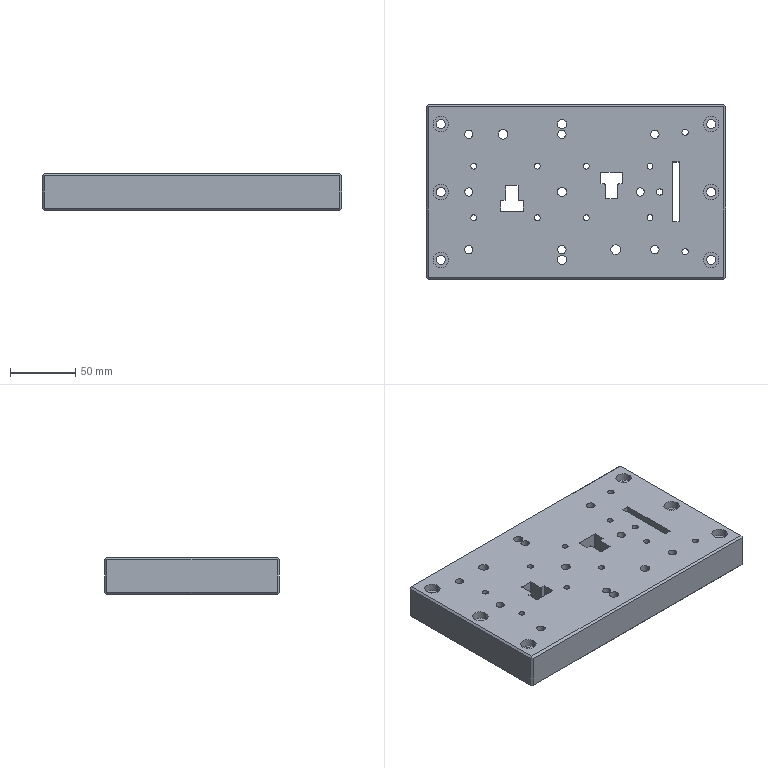Part | Creo | features CURVE 4, CUT 3, DATUM PLANE 3, CHAMFER 1, COORDINATE SYSTEM 1, PROTRUSION 1 | 1 solid | 132 faces | box 229.25 x 133.5 x 28 mm | volume 806588 mm3 | cylinder 88 | plane 44 | commonest cylinder face diameters 7 x18 0.76 x16 4.5 x16 6.38 x16 11.745 x12 4.88 x6